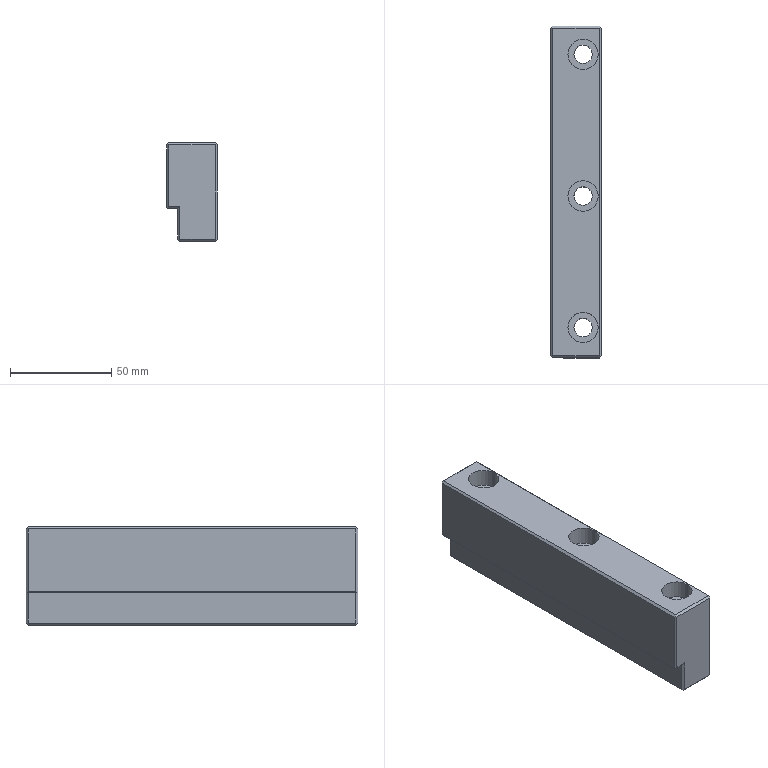Part | Creo | 1 solid | 40 faces | box 25 x 164 x 48.5 mm | volume 171619 mm3 | plane 28 | cylinder 12 | commonest cylinder face diameters 9 x6 15 x6
STEP:
#1=CARTESIAN_POINT('',(99.258,-211.005,-58.5));
#2=VERTEX_POINT('',#1);
#3=CARTESIAN_POINT('',(99.258,-211.005,-12.));
#4=VERTEX_POINT('',#3);
#5=CARTESIAN_POINT('',(99.258,-211.005,-58.5));
#6=DIRECTION('',(0.,0.,1.));
#7=VECTOR('',#6,46.5);
#8=LINE('',#5,#7);
#9=EDGE_CURVE('',#2,#4,#8,.T.);
#10=ORIENTED_EDGE('',*,*,#9,.T.);
#11=CARTESIAN_POINT('',(76.258,-211.005,-12.));
#12=VERTEX_POINT('',#11);
#13=CARTESIAN_POINT('',(99.258,-211.005,-12.));
#14=DIRECTION('',(-1.,0.,0.));
#15=VECTOR('',#14,23.);
#16=LINE('',#13,#15);
#17=EDGE_CURVE('',#4,#12,#16,.T.);
#18=ORIENTED_EDGE('',*,*,#17,.T.);
#19=CARTESIAN_POINT('',(76.258,-211.005,-42.5));
#20=VERTEX_POINT('',#19);
#21=CARTESIAN_POINT('',(76.258,-211.005,-12.));
#22=DIRECTION('',(0.,0.,-1.));
#23=VECTOR('',#22,30.5);
#24=LINE('',#21,#23);
#25=EDGE_CURVE('',#12,#20,#24,.T.);
#26=ORIENTED_EDGE('',*,*,#25,.T.);
#27=CARTESIAN_POINT('',(81.758,-211.005,-42.5));
#28=VERTEX_POINT('',#27);
#29=CARTESIAN_POINT('',(76.258,-211.005,-42.5));
#30=DIRECTION('',(1.,0.,0.));
#31=VECTOR('',#30,5.5);
#32=LINE('',#29,#31);
#33=EDGE_CURVE('',#20,#28,#32,.T.);
#34=ORIENTED_EDGE('',*,*,#33,.T.);
#35=CARTESIAN_POINT('',(81.758,-211.005,-58.5));
#36=VERTEX_POINT('',#35);
#37=CARTESIAN_POINT('',(81.758,-211.005,-42.5));
#38=DIRECTION('',(0.,0.,-1.));
#39=VECTOR('',#38,16.);
#40=LINE('',#37,#39);
#41=EDGE_CURVE('',#28,#36,#40,.T.);
#42=ORIENTED_EDGE('',*,*,#41,.T.);
#43=CARTESIAN_POINT('',(81.758,-211.005,-58.5));
#44=DIRECTION('',(1.,0.,0.));
#45=VECTOR('',#44,17.5);
#46=LINE('',#43,#45);
#47=EDGE_CURVE('',#36,#2,#46,.T.);
#48=ORIENTED_EDGE('',*,*,#47,.T.);
#49=EDGE_LOOP('',(#10,#18,#26,#34,#42,#48));
#50=FACE_OUTER_BOUND('',#49,.F.);
#51=CARTESIAN_POINT('',(-80.242,-211.005,-41.));
#52=DIRECTION('',(0.,1.,0.));
#53=DIRECTION('',(0.,0.,-1.));
#54=AXIS2_PLACEMENT_3D('',#51,#52,#53);
#55=PLANE('',#54);
#56=ADVANCED_FACE('',(#50),#55,.T.);
#57=CARTESIAN_POINT('',(100.258,-212.005,-12.));
#58=VERTEX_POINT('',#57);
#59=CARTESIAN_POINT('',(100.258,-212.005,-58.5));
#60=VERTEX_POINT('',#59);
#61=CARTESIAN_POINT('',(100.258,-212.005,-12.));
#62=DIRECTION('',(0.,0.,-1.));
#63=VECTOR('',#62,46.5);
#64=LINE('',#61,#63);
#65=EDGE_CURVE('',#58,#60,#64,.T.);
#66=ORIENTED_EDGE('',*,*,#65,.F.);
#67=CARTESIAN_POINT('',(99.758,-211.505,-11.5));
#68=VERTEX_POINT('',#67);
#69=CARTESIAN_POINT('',(99.758,-211.505,-11.5));
#70=DIRECTION('',(0.5774,-0.5774,-0.5774));
#71=VECTOR('',#70,0.866);
#72=LINE('',#69,#71);
#73=EDGE_CURVE('',#68,#58,#72,.T.);
#74=ORIENTED_EDGE('',*,*,#73,.F.);
#75=CARTESIAN_POINT('',(99.758,-211.505,-11.5));
#76=DIRECTION('',(-0.5774,0.5774,-0.5774));
#77=VECTOR('',#76,0.866);
#78=LINE('',#75,#77);
#79=EDGE_CURVE('',#68,#4,#78,.T.);
#80=ORIENTED_EDGE('',*,*,#79,.T.);
#81=ORIENTED_EDGE('',*,*,#9,.F.);
#82=CARTESIAN_POINT('',(99.758,-211.505,-59.));
#83=VERTEX_POINT('',#82);
#84=CARTESIAN_POINT('',(99.758,-211.505,-59.));
#85=DIRECTION('',(-0.5774,0.5774,0.5774));
#86=VECTOR('',#85,0.866);
#87=LINE('',#84,#86);
#88=EDGE_CURVE('',#83,#2,#87,.T.);
#89=ORIENTED_EDGE('',*,*,#88,.F.);
#90=CARTESIAN_POINT('',(100.258,-212.005,-58.5));
#91=DIRECTION('',(-0.5774,0.5774,-0.5774));
#92=VECTOR('',#91,0.866);
#93=LINE('',#90,#92);
#94=EDGE_CURVE('',#60,#83,#93,.T.);
#95=ORIENTED_EDGE('',*,*,#94,.F.);
#96=EDGE_LOOP('',(#66,#74,#80,#81,#89,#95));
#97=FACE_OUTER_BOUND('',#96,.F.);
#98=CARTESIAN_POINT('',(99.258,-211.005,-41.));
#99=DIRECTION('',(-0.7071,-0.7071,0.));
#100=DIRECTION('',(0.,0.,-1.));
#101=AXIS2_PLACEMENT_3D('',#98,#99,#100);
#102=PLANE('',#101);
#103=ADVANCED_FACE('',(#97),#102,.F.);
#104=CARTESIAN_POINT('',(100.258,-374.005,-58.5));
#105=VERTEX_POINT('',#104);
#106=CARTESIAN_POINT('',(100.258,-212.005,-58.5));
#107=DIRECTION('',(0.,-1.,0.));
#108=VECTOR('',#107,162.);
#109=LINE('',#106,#108);
#110=EDGE_CURVE('',#60,#105,#109,.T.);
#111=ORIENTED_EDGE('',*,*,#110,.T.);
#112=CARTESIAN_POINT('',(100.258,-374.005,-12.));
#113=VERTEX_POINT('',#112);
#114=CARTESIAN_POINT('',(100.258,-374.005,-12.));
#115=DIRECTION('',(0.,0.,-1.));
#116=VECTOR('',#115,46.5);
#117=LINE('',#114,#116);
#118=EDGE_CURVE('',#113,#105,#117,.T.);
#119=ORIENTED_EDGE('',*,*,#118,.F.);
#120=CARTESIAN_POINT('',(100.258,-212.005,-12.));
#121=DIRECTION('',(0.,-1.,0.));
#122=VECTOR('',#121,162.);
#123=LINE('',#120,#122);
#124=EDGE_CURVE('',#58,#113,#123,.T.);
#125=ORIENTED_EDGE('',*,*,#124,.F.);
#126=ORIENTED_EDGE('',*,*,#65,.T.);
#127=EDGE_LOOP('',(#111,#119,#125,#126));
#128=FACE_OUTER_BOUND('',#127,.F.);
#129=CARTESIAN_POINT('',(100.258,-210.005,-57.));
#130=DIRECTION('',(1.,0.,0.));
#131=DIRECTION('',(0.,0.,-1.));
#132=AXIS2_PLACEMENT_3D('',#129,#130,#131);
#133=PLANE('',#132);
#134=ADVANCED_FACE('',(#128),#133,.T.);
#135=CARTESIAN_POINT('',(99.258,-212.005,-59.5));
#136=VERTEX_POINT('',#135);
#137=CARTESIAN_POINT('',(99.758,-211.505,-59.));
#138=DIRECTION('',(-0.5774,-0.5774,-0.5774));
#139=VECTOR('',#138,0.866);
#140=LINE('',#137,#139);
#141=EDGE_CURVE('',#83,#136,#140,.T.);
#142=ORIENTED_EDGE('',*,*,#141,.T.);
#143=CARTESIAN_POINT('',(99.258,-374.005,-59.5));
#144=VERTEX_POINT('',#143);
#145=CARTESIAN_POINT('',(99.258,-212.005,-59.5));
#146=DIRECTION('',(0.,-1.,0.));
#147=VECTOR('',#146,162.);
#148=LINE('',#145,#147);
#149=EDGE_CURVE('',#136,#144,#148,.T.);
#150=ORIENTED_EDGE('',*,*,#149,.T.);
#151=CARTESIAN_POINT('',(99.758,-374.505,-59.));
#152=VERTEX_POINT('',#151);
#153=CARTESIAN_POINT('',(99.758,-374.505,-59.));
#154=DIRECTION('',(-0.5774,0.5774,-0.5774));
#155=VECTOR('',#154,0.866);
#156=LINE('',#153,#155);
#157=EDGE_CURVE('',#152,#144,#156,.T.);
#158=ORIENTED_EDGE('',*,*,#157,.F.);
#159=CARTESIAN_POINT('',(99.758,-374.505,-59.));
#160=DIRECTION('',(0.5774,0.5774,0.5774));
#161=VECTOR('',#160,0.866);
#162=LINE('',#159,#161);
#163=EDGE_CURVE('',#152,#105,#162,.T.);
#164=ORIENTED_EDGE('',*,*,#163,.T.);
#165=ORIENTED_EDGE('',*,*,#110,.F.);
#166=ORIENTED_EDGE('',*,*,#94,.T.);
#167=EDGE_LOOP('',(#142,#150,#158,#164,#165,#166));
#168=FACE_OUTER_BOUND('',#167,.F.);
#169=CARTESIAN_POINT('',(99.758,-280.005,-59.));
#170=DIRECTION('',(0.7071,0.,-0.7071));
#171=DIRECTION('',(0.7071,0.,0.7071));
#172=AXIS2_PLACEMENT_3D('',#169,#170,#171);
#173=PLANE('',#172);
#174=ADVANCED_FACE('',(#168),#173,.T.);
#175=CARTESIAN_POINT('',(81.758,-212.005,-59.5));
#176=VERTEX_POINT('',#175);
#177=CARTESIAN_POINT('',(99.258,-212.005,-59.5));
#178=DIRECTION('',(-1.,0.,0.));
#179=VECTOR('',#178,17.5);
#180=LINE('',#177,#179);
#181=EDGE_CURVE('',#136,#176,#180,.T.);
#182=ORIENTED_EDGE('',*,*,#181,.F.);
#183=ORIENTED_EDGE('',*,*,#141,.F.);
#184=ORIENTED_EDGE('',*,*,#88,.T.);
#185=ORIENTED_EDGE('',*,*,#47,.F.);
#186=CARTESIAN_POINT('',(81.258,-211.505,-59.));
#187=VERTEX_POINT('',#186);
#188=CARTESIAN_POINT('',(81.258,-211.505,-59.));
#189=DIRECTION('',(0.5774,0.5774,0.5774));
#190=VECTOR('',#189,0.866);
#191=LINE('',#188,#190);
#192=EDGE_CURVE('',#187,#36,#191,.T.);
#193=ORIENTED_EDGE('',*,*,#192,.F.);
#194=CARTESIAN_POINT('',(81.758,-212.005,-59.5));
#195=DIRECTION('',(-0.5774,0.5774,0.5774));
#196=VECTOR('',#195,0.866);
#197=LINE('',#194,#196);
#198=EDGE_CURVE('',#176,#187,#197,.T.);
#199=ORIENTED_EDGE('',*,*,#198,.F.);
#200=EDGE_LOOP('',(#182,#183,#184,#185,#193,#199));
#201=FACE_OUTER_BOUND('',#200,.F.);
#202=CARTESIAN_POINT('',(-80.242,-211.005,-58.5));
#203=DIRECTION('',(0.,-0.7071,0.7071));
#204=DIRECTION('',(-1.,0.,0.));
#205=AXIS2_PLACEMENT_3D('',#202,#203,#204);
#206=PLANE('',#205);
#207=ADVANCED_FACE('',(#201),#206,.F.);
#208=CARTESIAN_POINT('',(81.758,-374.005,-59.5));
#209=VERTEX_POINT('',#208);
#210=CARTESIAN_POINT('',(81.758,-212.005,-59.5));
#211=DIRECTION('',(0.,-1.,0.));
#212=VECTOR('',#211,162.);
#213=LINE('',#210,#212);
#214=EDGE_CURVE('',#176,#209,#213,.T.);
#215=ORIENTED_EDGE('',*,*,#214,.T.);
#216=CARTESIAN_POINT('',(99.258,-374.005,-59.5));
#217=DIRECTION('',(-1.,0.,0.));
#218=VECTOR('',#217,17.5);
#219=LINE('',#216,#218);
#220=EDGE_CURVE('',#144,#209,#219,.T.);
#221=ORIENTED_EDGE('',*,*,#220,.F.);
#222=ORIENTED_EDGE('',*,*,#149,.F.);
#223=ORIENTED_EDGE('',*,*,#181,.T.);
#224=EDGE_LOOP('',(#215,#221,#222,#223));
#225=FACE_OUTER_BOUND('',#224,.F.);
#226=CARTESIAN_POINT('',(86.758,-360.005,-59.5));
#227=VERTEX_POINT('',#226);
#228=CARTESIAN_POINT('',(95.758,-360.005,-59.5));
#229=VERTEX_POINT('',#228);
#230=CARTESIAN_POINT('',(91.258,-360.005,-59.5));
#231=DIRECTION('',(0.,0.,1.));
#232=DIRECTION('',(-1.,0.,0.));
#233=AXIS2_PLACEMENT_3D('',#230,#231,#232);
#234=CIRCLE('',#233,4.5);
#235=EDGE_CURVE('',#227,#229,#234,.T.);
#236=ORIENTED_EDGE('',*,*,#235,.F.);
#237=CARTESIAN_POINT('',(91.258,-360.005,-59.5));
#238=DIRECTION('',(0.,0.,1.));
#239=DIRECTION('',(1.,0.,0.));
#240=AXIS2_PLACEMENT_3D('',#237,#238,#239);
#241=CIRCLE('',#240,4.5);
#242=EDGE_CURVE('',#229,#227,#241,.T.);
#243=ORIENTED_EDGE('',*,*,#242,.F.);
#244=EDGE_LOOP('',(#236,#243));
#245=FACE_BOUND('',#244,.F.);
#246=CARTESIAN_POINT('',(86.758,-225.005,-59.5));
#247=VERTEX_POINT('',#246);
#248=CARTESIAN_POINT('',(95.758,-225.005,-59.5));
#249=VERTEX_POINT('',#248);
#250=CARTESIAN_POINT('',(91.258,-225.005,-59.5));
#251=DIRECTION('',(0.,0.,1.));
#252=DIRECTION('',(-1.,0.,0.));
#253=AXIS2_PLACEMENT_3D('',#250,#251,#252);
#254=CIRCLE('',#253,4.5);
#255=EDGE_CURVE('',#247,#249,#254,.T.);
#256=ORIENTED_EDGE('',*,*,#255,.F.);
#257=CARTESIAN_POINT('',(91.258,-225.005,-59.5));
#258=DIRECTION('',(0.,0.,1.));
#259=DIRECTION('',(1.,0.,0.));
#260=AXIS2_PLACEMENT_3D('',#257,#258,#259);
#261=CIRCLE('',#260,4.5);
#262=EDGE_CURVE('',#249,#247,#261,.T.);
#263=ORIENTED_EDGE('',*,*,#262,.F.);
#264=EDGE_LOOP('',(#256,#263));
#265=FACE_BOUND('',#264,.F.);
#266=CARTESIAN_POINT('',(86.758,-295.005,-59.5));
#267=VERTEX_POINT('',#266);
#268=CARTESIAN_POINT('',(95.758,-295.005,-59.5));
#269=VERTEX_POINT('',#268);
#270=CARTESIAN_POINT('',(91.258,-295.005,-59.5));
#271=DIRECTION('',(0.,0.,1.));
#272=DIRECTION('',(-1.,0.,0.));
#273=AXIS2_PLACEMENT_3D('',#270,#271,#272);
#274=CIRCLE('',#273,4.5);
#275=EDGE_CURVE('',#267,#269,#274,.T.);
#276=ORIENTED_EDGE('',*,*,#275,.F.);
#277=CARTESIAN_POINT('',(91.258,-295.005,-59.5));
#278=DIRECTION('',(0.,0.,1.));
#279=DIRECTION('',(1.,0.,0.));
#280=AXIS2_PLACEMENT_3D('',#277,#278,#279);
#281=CIRCLE('',#280,4.5);
#282=EDGE_CURVE('',#269,#267,#281,.T.);
#283=ORIENTED_EDGE('',*,*,#282,.F.);
#284=EDGE_LOOP('',(#276,#283));
#285=FACE_BOUND('',#284,.F.);
#286=CARTESIAN_POINT('',(80.758,-210.005,-59.5));
#287=DIRECTION('',(0.,0.,-1.));
#288=DIRECTION('',(-1.,0.,0.));
#289=AXIS2_PLACEMENT_3D('',#286,#287,#288);
#290=PLANE('',#289);
#291=ADVANCED_FACE('',(#225,#245,#265,#285),#290,.T.);
#292=CARTESIAN_POINT('',(95.758,-295.005,-20.));
#293=VERTEX_POINT('',#292);
#294=CARTESIAN_POINT('',(86.758,-295.005,-20.));
#295=VERTEX_POINT('',#294);
#296=CARTESIAN_POINT('',(91.258,-295.005,-20.));
#297=DIRECTION('',(0.,0.,-1.));
#298=DIRECTION('',(1.,0.,0.));
#299=AXIS2_PLACEMENT_3D('',#296,#297,#298);
#300=CIRCLE('',#299,4.5);
#301=EDGE_CURVE('',#293,#295,#300,.T.);
#302=ORIENTED_EDGE('',*,*,#301,.T.);
#303=CARTESIAN_POINT('',(86.758,-295.005,-59.5));
#304=DIRECTION('',(0.,0.,1.));
#305=VECTOR('',#304,39.5);
#306=LINE('',#303,#305);
#307=EDGE_CURVE('',#267,#295,#306,.T.);
#308=ORIENTED_EDGE('',*,*,#307,.F.);
#309=ORIENTED_EDGE('',*,*,#275,.T.);
#310=CARTESIAN_POINT('',(95.758,-295.005,-59.5));
#311=DIRECTION('',(0.,0.,1.));
#312=VECTOR('',#311,39.5);
#313=LINE('',#310,#312);
#314=EDGE_CURVE('',#269,#293,#313,.T.);
#315=ORIENTED_EDGE('',*,*,#314,.T.);
#316=EDGE_LOOP('',(#302,#308,#309,#315));
#317=FACE_OUTER_BOUND('',#316,.F.);
#318=CARTESIAN_POINT('',(91.258,-295.005,-10.));
#319=DIRECTION('',(0.,0.,1.));
#320=DIRECTION('',(-1.,0.,0.));
#321=AXIS2_PLACEMENT_3D('',#318,#319,#320);
#322=CYLINDRICAL_SURFACE('',#321,4.5);
#323=ADVANCED_FACE('',(#317),#322,.F.);
#324=CARTESIAN_POINT('',(98.758,-295.005,-20.));
#325=VERTEX_POINT('',#324);
#326=CARTESIAN_POINT('',(83.758,-295.005,-20.));
#327=VERTEX_POINT('',#326);
#328=CARTESIAN_POINT('',(91.258,-295.005,-20.));
#329=DIRECTION('',(0.,0.,1.));
#330=DIRECTION('',(1.,0.,0.));
#331=AXIS2_PLACEMENT_3D('',#328,#329,#330);
#332=CIRCLE('',#331,7.5);
#333=EDGE_CURVE('',#325,#327,#332,.T.);
#334=ORIENTED_EDGE('',*,*,#333,.F.);
#335=CARTESIAN_POINT('',(91.258,-295.005,-20.));
#336=DIRECTION('',(0.,0.,1.));
#337=DIRECTION('',(-1.,0.,0.));
#338=AXIS2_PLACEMENT_3D('',#335,#336,#337);
#339=CIRCLE('',#338,7.5);
#340=EDGE_CURVE('',#327,#325,#339,.T.);
#341=ORIENTED_EDGE('',*,*,#340,.F.);
#342=EDGE_LOOP('',(#334,#341));
#343=FACE_OUTER_BOUND('',#342,.F.);
#344=CARTESIAN_POINT('',(91.258,-295.005,-20.));
#345=DIRECTION('',(0.,0.,-1.));
#346=DIRECTION('',(-1.,0.,0.));
#347=AXIS2_PLACEMENT_3D('',#344,#345,#346);
#348=CIRCLE('',#347,4.5);
#349=EDGE_CURVE('',#295,#293,#348,.T.);
#350=ORIENTED_EDGE('',*,*,#349,.F.);
#351=ORIENTED_EDGE('',*,*,#301,.F.);
#352=EDGE_LOOP('',(#350,#351));
#353=FACE_BOUND('',#352,.F.);
#354=CARTESIAN_POINT('',(91.258,-295.005,-20.));
#355=DIRECTION('',(0.,0.,-1.));
#356=DIRECTION('',(-1.,0.,0.));
#357=AXIS2_PLACEMENT_3D('',#354,#355,#356);
#358=PLANE('',#357);
#359=ADVANCED_FACE('',(#343,#353),#358,.F.);
#360=ORIENTED_EDGE('',*,*,#349,.T.);
#361=ORIENTED_EDGE('',*,*,#314,.F.);
#362=ORIENTED_EDGE('',*,*,#282,.T.);
#363=ORIENTED_EDGE('',*,*,#307,.T.);
#364=EDGE_LOOP('',(#360,#361,#362,#363));
#365=FACE_OUTER_BOUND('',#364,.F.);
#366=CARTESIAN_POINT('',(91.258,-295.005,-10.));
#367=DIRECTION('',(0.,0.,1.));
#368=DIRECTION('',(-1.,0.,0.));
#369=AXIS2_PLACEMENT_3D('',#366,#367,#368);
#370=CYLINDRICAL_SURFACE('',#369,4.5);
#371=ADVANCED_FACE('',(#365),#370,.F.);
#372=ORIENTED_EDGE('',*,*,#333,.T.);
#373=CARTESIAN_POINT('',(83.758,-295.005,-11.));
#374=VERTEX_POINT('',#373);
#375=CARTESIAN_POINT('',(83.758,-295.005,-11.));
#376=DIRECTION('',(0.,0.,-1.));
#377=VECTOR('',#376,9.);
#378=LINE('',#375,#377);
#379=EDGE_CURVE('',#374,#327,#378,.T.);
#380=ORIENTED_EDGE('',*,*,#379,.F.);
#381=CARTESIAN_POINT('',(98.758,-295.005,-11.));
#382=VERTEX_POINT('',#381);
#383=CARTESIAN_POINT('',(91.258,-295.005,-11.));
#384=DIRECTION('',(0.,0.,-1.));
#385=DIRECTION('',(-1.,0.,0.));
#386=AXIS2_PLACEMENT_3D('',#383,#384,#385);
#387=CIRCLE('',#386,7.5);
#388=EDGE_CURVE('',#374,#382,#387,.T.);
#389=ORIENTED_EDGE('',*,*,#388,.T.);
#390=CARTESIAN_POINT('',(98.758,-295.005,-11.));
#391=DIRECTION('',(0.,0.,-1.));
#392=VECTOR('',#391,9.);
#393=LINE('',#390,#392);
#394=EDGE_CURVE('',#382,#325,#393,.T.);
#395=ORIENTED_EDGE('',*,*,#394,.T.);
#396=EDGE_LOOP('',(#372,#380,#389,#395));
#397=FACE_OUTER_BOUND('',#396,.F.);
#398=CARTESIAN_POINT('',(91.258,-295.005,-10.55));
#399=DIRECTION('',(0.,0.,-1.));
#400=DIRECTION('',(-1.,0.,0.));
#401=AXIS2_PLACEMENT_3D('',#398,#399,#400);
#402=CYLINDRICAL_SURFACE('',#401,7.5);
#403=ADVANCED_FACE('',(#397),#402,.F.);
#404=ORIENTED_EDGE('',*,*,#340,.T.);
#405=ORIENTED_EDGE('',*,*,#394,.F.);
#406=CARTESIAN_POINT('',(91.258,-295.005,-11.));
#407=DIRECTION('',(0.,0.,-1.));
#408=DIRECTION('',(1.,0.,0.));
#409=AXIS2_PLACEMENT_3D('',#406,#407,#408);
#410=CIRCLE('',#409,7.5);
#411=EDGE_CURVE('',#382,#374,#410,.T.);
#412=ORIENTED_EDGE('',*,*,#411,.T.);
#413=ORIENTED_EDGE('',*,*,#379,.T.);
#414=EDGE_LOOP('',(#404,#405,#412,#413));
#415=FACE_OUTER_BOUND('',#414,.F.);
#416=CARTESIAN_POINT('',(91.258,-295.005,-10.55));
#417=DIRECTION('',(0.,0.,-1.));
#418=DIRECTION('',(-1.,0.,0.));
#419=AXIS2_PLACEMENT_3D('',#416,#417,#418);
#420=CYLINDRICAL_SURFACE('',#419,7.5);
#421=ADVANCED_FACE('',(#415),#420,.F.);
#422=CARTESIAN_POINT('',(99.258,-212.005,-11.));
#423=VERTEX_POINT('',#422);
#424=CARTESIAN_POINT('',(99.258,-374.005,-11.));
#425=VERTEX_POINT('',#424);
#426=CARTESIAN_POINT('',(99.258,-212.005,-11.));
#427=DIRECTION('',(0.,-1.,0.));
#428=VECTOR('',#427,162.);
#429=LINE('',#426,#428);
#430=EDGE_CURVE('',#423,#425,#429,.T.);
#431=ORIENTED_EDGE('',*,*,#430,.T.);
#432=CARTESIAN_POINT('',(76.258,-374.005,-11.));
#433=VERTEX_POINT('',#432);
#434=CARTESIAN_POINT('',(76.258,-374.005,-11.));
#435=DIRECTION('',(1.,0.,0.));
#436=VECTOR('',#435,23.);
#437=LINE('',#434,#436);
#438=EDGE_CURVE('',#433,#425,#437,.T.);
#439=ORIENTED_EDGE('',*,*,#438,.F.);
#440=CARTESIAN_POINT('',(76.258,-212.005,-11.));
#441=VERTEX_POINT('',#440);
#442=CARTESIAN_POINT('',(76.258,-212.005,-11.));
#443=DIRECTION('',(0.,-1.,0.));
#444=VECTOR('',#443,162.);
#445=LINE('',#442,#444);
#446=EDGE_CURVE('',#441,#433,#445,.T.);
#447=ORIENTED_EDGE('',*,*,#446,.F.);
#448=CARTESIAN_POINT('',(76.258,-212.005,-11.));
#449=DIRECTION('',(1.,0.,0.));
#450=VECTOR('',#449,23.);
#451=LINE('',#448,#450);
#452=EDGE_CURVE('',#441,#423,#451,.T.);
#453=ORIENTED_EDGE('',*,*,#452,.T.);
#454=EDGE_LOOP('',(#431,#439,#447,#453));
#455=FACE_OUTER_BOUND('',#454,.F.);
#456=CARTESIAN_POINT('',(83.758,-360.005,-11.));
#457=VERTEX_POINT('',#456);
#458=CARTESIAN_POINT('',(98.758,-360.005,-11.));
#459=VERTEX_POINT('',#458);
#460=CARTESIAN_POINT('',(91.258,-360.005,-11.));
#461=DIRECTION('',(0.,0.,-1.));
#462=DIRECTION('',(-1.,0.,0.));
#463=AXIS2_PLACEMENT_3D('',#460,#461,#462);
#464=CIRCLE('',#463,7.5);
#465=EDGE_CURVE('',#457,#459,#464,.T.);
#466=ORIENTED_EDGE('',*,*,#465,.F.);
#467=CARTESIAN_POINT('',(91.258,-360.005,-11.));
#468=DIRECTION('',(0.,0.,-1.));
#469=DIRECTION('',(1.,0.,0.));
#470=AXIS2_PLACEMENT_3D('',#467,#468,#469);
#471=CIRCLE('',#470,7.5);
#472=EDGE_CURVE('',#459,#457,#471,.T.);
#473=ORIENTED_EDGE('',*,*,#472,.F.);
#474=EDGE_LOOP('',(#466,#473));
#475=FACE_BOUND('',#474,.F.);
#476=CARTESIAN_POINT('',(83.758,-225.005,-11.));
#477=VERTEX_POINT('',#476);
#478=CARTESIAN_POINT('',(98.758,-225.005,-11.));
#479=VERTEX_POINT('',#478);
#480=CARTESIAN_POINT('',(91.258,-225.005,-11.));
#481=DIRECTION('',(0.,0.,-1.));
#482=DIRECTION('',(-1.,0.,0.));
#483=AXIS2_PLACEMENT_3D('',#480,#481,#482);
#484=CIRCLE('',#483,7.5);
#485=EDGE_CURVE('',#477,#479,#484,.T.);
#486=ORIENTED_EDGE('',*,*,#485,.F.);
#487=CARTESIAN_POINT('',(91.258,-225.005,-11.));
#488=DIRECTION('',(0.,0.,-1.));
#489=DIRECTION('',(1.,0.,0.));
#490=AXIS2_PLACEMENT_3D('',#487,#488,#489);
#491=CIRCLE('',#490,7.5);
#492=EDGE_CURVE('',#479,#477,#491,.T.);
#493=ORIENTED_EDGE('',*,*,#492,.F.);
#494=EDGE_LOOP('',(#486,#493));
#495=FACE_BOUND('',#494,.F.);
#496=ORIENTED_EDGE('',*,*,#388,.F.);
#497=ORIENTED_EDGE('',*,*,#411,.F.);
#498=EDGE_LOOP('',(#496,#497));
#499=FACE_BOUND('',#498,.F.);
#500=CARTESIAN_POINT('',(100.258,-210.005,-11.));
#501=DIRECTION('',(0.,0.,1.));
#502=DIRECTION('',(1.,0.,0.));
#503=AXIS2_PLACEMENT_3D('',#500,#501,#502);
#504=PLANE('',#503);
#505=ADVANCED_FACE('',(#455,#475,#495,#499),#504,.T.);
#506=CARTESIAN_POINT('',(98.758,-360.005,-20.));
#507=VERTEX_POINT('',#506);
#508=CARTESIAN_POINT('',(83.758,-360.005,-20.));
#509=VERTEX_POINT('',#508);
#510=CARTESIAN_POINT('',(91.258,-360.005,-20.));
#511=DIRECTION('',(0.,0.,1.));
#512=DIRECTION('',(1.,0.,0.));
#513=AXIS2_PLACEMENT_3D('',#510,#511,#512);
#514=CIRCLE('',#513,7.5);
#515=EDGE_CURVE('',#507,#509,#514,.T.);
#516=ORIENTED_EDGE('',*,*,#515,.T.);
#517=CARTESIAN_POINT('',(83.758,-360.005,-11.));
#518=DIRECTION('',(0.,0.,-1.));
#519=VECTOR('',#518,9.);
#520=LINE('',#517,#519);
#521=EDGE_CURVE('',#457,#509,#520,.T.);
#522=ORIENTED_EDGE('',*,*,#521,.F.);
#523=ORIENTED_EDGE('',*,*,#465,.T.);
#524=CARTESIAN_POINT('',(98.758,-360.005,-11.));
#525=DIRECTION('',(0.,0.,-1.));
#526=VECTOR('',#525,9.);
#527=LINE('',#524,#526);
#528=EDGE_CURVE('',#459,#507,#527,.T.);
#529=ORIENTED_EDGE('',*,*,#528,.T.);
#530=EDGE_LOOP('',(#516,#522,#523,#529));
#531=FACE_OUTER_BOUND('',#530,.F.);
#532=CARTESIAN_POINT('',(91.258,-360.005,-10.55));
#533=DIRECTION('',(0.,0.,-1.));
#534=DIRECTION('',(-1.,0.,0.));
#535=AXIS2_PLACEMENT_3D('',#532,#533,#534);
#536=CYLINDRICAL_SURFACE('',#535,7.5);
#537=ADVANCED_FACE('',(#531),#536,.F.);
#538=ORIENTED_EDGE('',*,*,#515,.F.);
#539=CARTESIAN_POINT('',(91.258,-360.005,-20.));
#540=DIRECTION('',(0.,0.,1.));
#541=DIRECTION('',(-1.,0.,0.));
#542=AXIS2_PLACEMENT_3D('',#539,#540,#541);
#543=CIRCLE('',#542,7.5);
#544=EDGE_CURVE('',#509,#507,#543,.T.);
#545=ORIENTED_EDGE('',*,*,#544,.F.);
#546=EDGE_LOOP('',(#538,#545));
#547=FACE_OUTER_BOUND('',#546,.F.);
#548=CARTESIAN_POINT('',(86.758,-360.005,-20.));
#549=VERTEX_POINT('',#548);
#550=CARTESIAN_POINT('',(95.758,-360.005,-20.));
#551=VERTEX_POINT('',#550);
#552=CARTESIAN_POINT('',(91.258,-360.005,-20.));
#553=DIRECTION('',(0.,0.,-1.));
#554=DIRECTION('',(-1.,0.,0.));
#555=AXIS2_PLACEMENT_3D('',#552,#553,#554);
#556=CIRCLE('',#555,4.5);
#557=EDGE_CURVE('',#549,#551,#556,.T.);
#558=ORIENTED_EDGE('',*,*,#557,.F.);
#559=CARTESIAN_POINT('',(91.258,-360.005,-20.));
#560=DIRECTION('',(0.,0.,-1.));
#561=DIRECTION('',(1.,0.,0.));
#562=AXIS2_PLACEMENT_3D('',#559,#560,#561);
#563=CIRCLE('',#562,4.5);
#564=EDGE_CURVE('',#551,#549,#563,.T.);
#565=ORIENTED_EDGE('',*,*,#564,.F.);
#566=EDGE_LOOP('',(#558,#565));
#567=FACE_BOUND('',#566,.F.);
#568=CARTESIAN_POINT('',(91.258,-360.005,-20.));
#569=DIRECTION('',(0.,0.,-1.));
#570=DIRECTION('',(-1.,0.,0.));
#571=AXIS2_PLACEMENT_3D('',#568,#569,#570);
#572=PLANE('',#571);
#573=ADVANCED_FACE('',(#547,#567),#572,.F.);
#574=ORIENTED_EDGE('',*,*,#557,.T.);
#575=CARTESIAN_POINT('',(95.758,-360.005,-59.5));
#576=DIRECTION('',(0.,0.,1.));
#577=VECTOR('',#576,39.5);
#578=LINE('',#575,#577);
#579=EDGE_CURVE('',#229,#551,#578,.T.);
#580=ORIENTED_EDGE('',*,*,#579,.F.);
#581=ORIENTED_EDGE('',*,*,#242,.T.);
#582=CARTESIAN_POINT('',(86.758,-360.005,-59.5));
#583=DIRECTION('',(0.,0.,1.));
#584=VECTOR('',#583,39.5);
#585=LINE('',#582,#584);
#586=EDGE_CURVE('',#227,#549,#585,.T.);
#587=ORIENTED_EDGE('',*,*,#586,.T.);
#588=EDGE_LOOP('',(#574,#580,#581,#587));
#589=FACE_OUTER_BOUND('',#588,.F.);
#590=CARTESIAN_POINT('',(91.258,-360.005,-10.));
#591=DIRECTION('',(0.,0.,1.));
#592=DIRECTION('',(-1.,0.,0.));
#593=AXIS2_PLACEMENT_3D('',#590,#591,#592);
#594=CYLINDRICAL_SURFACE('',#593,4.5);
#595=ADVANCED_FACE('',(#589),#594,.F.);
#596=ORIENTED_EDGE('',*,*,#564,.T.);
#597=ORIENTED_EDGE('',*,*,#586,.F.);
#598=ORIENTED_EDGE('',*,*,#235,.T.);
#599=ORIENTED_EDGE('',*,*,#579,.T.);
#600=EDGE_LOOP('',(#596,#597,#598,#599));
#601=FACE_OUTER_BOUND('',#600,.F.);
#602=CARTESIAN_POINT('',(91.258,-360.005,-10.));
#603=DIRECTION('',(0.,0.,1.));
#604=DIRECTION('',(-1.,0.,0.));
#605=AXIS2_PLACEMENT_3D('',#602,#603,#604);
#606=CYLINDRICAL_SURFACE('',#605,4.5);
#607=ADVANCED_FACE('',(#601),#606,.F.);
#608=ORIENTED_EDGE('',*,*,#544,.T.);
#609=ORIENTED_EDGE('',*,*,#528,.F.);
#610=ORIENTED_EDGE('',*,*,#472,.T.);
#611=ORIENTED_EDGE('',*,*,#521,.T.);
#612=EDGE_LOOP('',(#608,#609,#610,#611));
#613=FACE_OUTER_BOUND('',#612,.F.);
#614=CARTESIAN_POINT('',(91.258,-360.005,-10.55));
#615=DIRECTION('',(0.,0.,-1.));
#616=DIRECTION('',(-1.,0.,0.));
#617=AXIS2_PLACEMENT_3D('',#614,#615,#616);
#618=CYLINDRICAL_SURFACE('',#617,7.5);
#619=ADVANCED_FACE('',(#613),#618,.F.);
#620=CARTESIAN_POINT('',(98.758,-225.005,-20.));
#621=VERTEX_POINT('',#620);
#622=CARTESIAN_POINT('',(83.758,-225.005,-20.));
#623=VERTEX_POINT('',#622);
#624=CARTESIAN_POINT('',(91.258,-225.005,-20.));
#625=DIRECTION('',(0.,0.,1.));
#626=DIRECTION('',(1.,0.,0.));
#627=AXIS2_PLACEMENT_3D('',#624,#625,#626);
#628=CIRCLE('',#627,7.5);
#629=EDGE_CURVE('',#621,#623,#628,.T.);
#630=ORIENTED_EDGE('',*,*,#629,.T.);
#631=CARTESIAN_POINT('',(83.758,-225.005,-11.));
#632=DIRECTION('',(0.,0.,-1.));
#633=VECTOR('',#632,9.);
#634=LINE('',#631,#633);
#635=EDGE_CURVE('',#477,#623,#634,.T.);
#636=ORIENTED_EDGE('',*,*,#635,.F.);
#637=ORIENTED_EDGE('',*,*,#485,.T.);
#638=CARTESIAN_POINT('',(98.758,-225.005,-11.));
#639=DIRECTION('',(0.,0.,-1.));
#640=VECTOR('',#639,9.);
#641=LINE('',#638,#640);
#642=EDGE_CURVE('',#479,#621,#641,.T.);
#643=ORIENTED_EDGE('',*,*,#642,.T.);
#644=EDGE_LOOP('',(#630,#636,#637,#643));
#645=FACE_OUTER_BOUND('',#644,.F.);
#646=CARTESIAN_POINT('',(91.258,-225.005,-10.55));
#647=DIRECTION('',(0.,0.,-1.));
#648=DIRECTION('',(-1.,0.,0.));
#649=AXIS2_PLACEMENT_3D('',#646,#647,#648);
#650=CYLINDRICAL_SURFACE('',#649,7.5);
#651=ADVANCED_FACE('',(#645),#650,.F.);
#652=ORIENTED_EDGE('',*,*,#629,.F.);
#653=CARTESIAN_POINT('',(91.258,-225.005,-20.));
#654=DIRECTION('',(0.,0.,1.));
#655=DIRECTION('',(-1.,0.,0.));
#656=AXIS2_PLACEMENT_3D('',#653,#654,#655);
#657=CIRCLE('',#656,7.5);
#658=EDGE_CURVE('',#623,#621,#657,.T.);
#659=ORIENTED_EDGE('',*,*,#658,.F.);
#660=EDGE_LOOP('',(#652,#659));
#661=FACE_OUTER_BOUND('',#660,.F.);
#662=CARTESIAN_POINT('',(86.758,-225.005,-20.));
#663=VERTEX_POINT('',#662);
#664=CARTESIAN_POINT('',(95.758,-225.005,-20.));
#665=VERTEX_POINT('',#664);
#666=CARTESIAN_POINT('',(91.258,-225.005,-20.));
#667=DIRECTION('',(0.,0.,-1.));
#668=DIRECTION('',(-1.,0.,0.));
#669=AXIS2_PLACEMENT_3D('',#666,#667,#668);
#670=CIRCLE('',#669,4.5);
#671=EDGE_CURVE('',#663,#665,#670,.T.);
#672=ORIENTED_EDGE('',*,*,#671,.F.);
#673=CARTESIAN_POINT('',(91.258,-225.005,-20.));
#674=DIRECTION('',(0.,0.,-1.));
#675=DIRECTION('',(1.,0.,0.));
#676=AXIS2_PLACEMENT_3D('',#673,#674,#675);
#677=CIRCLE('',#676,4.5);
#678=EDGE_CURVE('',#665,#663,#677,.T.);
#679=ORIENTED_EDGE('',*,*,#678,.F.);
#680=EDGE_LOOP('',(#672,#679));
#681=FACE_BOUND('',#680,.F.);
#682=CARTESIAN_POINT('',(91.258,-225.005,-20.));
#683=DIRECTION('',(0.,0.,-1.));
#684=DIRECTION('',(-1.,0.,0.));
#685=AXIS2_PLACEMENT_3D('',#682,#683,#684);
#686=PLANE('',#685);
#687=ADVANCED_FACE('',(#661,#681),#686,.F.);
#688=ORIENTED_EDGE('',*,*,#671,.T.);
#689=CARTESIAN_POINT('',(95.758,-225.005,-59.5));
#690=DIRECTION('',(0.,0.,1.));
#691=VECTOR('',#690,39.5);
#692=LINE('',#689,#691);
#693=EDGE_CURVE('',#249,#665,#692,.T.);
#694=ORIENTED_EDGE('',*,*,#693,.F.);
#695=ORIENTED_EDGE('',*,*,#262,.T.);
#696=CARTESIAN_POINT('',(86.758,-225.005,-59.5));
#697=DIRECTION('',(0.,0.,1.));
#698=VECTOR('',#697,39.5);
#699=LINE('',#696,#698);
#700=EDGE_CURVE('',#247,#663,#699,.T.);
#701=ORIENTED_EDGE('',*,*,#700,.T.);
#702=EDGE_LOOP('',(#688,#694,#695,#701));
#703=FACE_OUTER_BOUND('',#702,.F.);
#704=CARTESIAN_POINT('',(91.258,-225.005,-10.));
#705=DIRECTION('',(0.,0.,1.));
#706=DIRECTION('',(-1.,0.,0.));
#707=AXIS2_PLACEMENT_3D('',#704,#705,#706);
#708=CYLINDRICAL_SURFACE('',#707,4.5);
#709=ADVANCED_FACE('',(#703),#708,.F.);
#710=ORIENTED_EDGE('',*,*,#678,.T.);
#711=ORIENTED_EDGE('',*,*,#700,.F.);
#712=ORIENTED_EDGE('',*,*,#255,.T.);
#713=ORIENTED_EDGE('',*,*,#693,.T.);
#714=EDGE_LOOP('',(#710,#711,#712,#713));
#715=FACE_OUTER_BOUND('',#714,.F.);
#716=CARTESIAN_POINT('',(91.258,-225.005,-10.));
#717=DIRECTION('',(0.,0.,1.));
#718=DIRECTION('',(-1.,0.,0.));
#719=AXIS2_PLACEMENT_3D('',#716,#717,#718);
#720=CYLINDRICAL_SURFACE('',#719,4.5);
#721=ADVANCED_FACE('',(#715),#720,.F.);
#722=ORIENTED_EDGE('',*,*,#658,.T.);
#723=ORIENTED_EDGE('',*,*,#642,.F.);
#724=ORIENTED_EDGE('',*,*,#492,.T.);
#725=ORIENTED_EDGE('',*,*,#635,.T.);
#726=EDGE_LOOP('',(#722,#723,#724,#725));
#727=FACE_OUTER_BOUND('',#726,.F.);
#728=CARTESIAN_POINT('',(91.258,-225.005,-10.55));
#729=DIRECTION('',(0.,0.,-1.));
#730=DIRECTION('',(-1.,0.,0.));
#731=AXIS2_PLACEMENT_3D('',#728,#729,#730);
#732=CYLINDRICAL_SURFACE('',#731,7.5);
#733=ADVANCED_FACE('',(#727),#732,.F.);
#734=ORIENTED_EDGE('',*,*,#124,.T.);
#735=CARTESIAN_POINT('',(99.758,-374.505,-11.5));
#736=VERTEX_POINT('',#735);
#737=CARTESIAN_POINT('',(100.258,-374.005,-12.));
#738=DIRECTION('',(-0.5774,-0.5774,0.5774));
#739=VECTOR('',#738,0.866);
#740=LINE('',#737,#739);
#741=EDGE_CURVE('',#113,#736,#740,.T.);
#742=ORIENTED_EDGE('',*,*,#741,.T.);
#743=CARTESIAN_POINT('',(99.758,-374.505,-11.5));
#744=DIRECTION('',(-0.5774,0.5774,0.5774));
#745=VECTOR('',#744,0.866);
#746=LINE('',#743,#745);
#747=EDGE_CURVE('',#736,#425,#746,.T.);
#748=ORIENTED_EDGE('',*,*,#747,.T.);
#749=ORIENTED_EDGE('',*,*,#430,.F.);
#750=CARTESIAN_POINT('',(99.258,-212.005,-11.));
#751=DIRECTION('',(0.5774,0.5774,-0.5774));
#752=VECTOR('',#751,0.866);
#753=LINE('',#750,#752);
#754=EDGE_CURVE('',#423,#68,#753,.T.);
#755=ORIENTED_EDGE('',*,*,#754,.T.);
#756=ORIENTED_EDGE('',*,*,#73,.T.);
#757=EDGE_LOOP('',(#734,#742,#748,#749,#755,#756));
#758=FACE_OUTER_BOUND('',#757,.F.);
#759=CARTESIAN_POINT('',(99.758,-280.005,-11.5));
#760=DIRECTION('',(0.7071,0.,0.7071));
#761=DIRECTION('',(-0.7071,0.,0.7071));
#762=AXIS2_PLACEMENT_3D('',#759,#760,#761);
#763=PLANE('',#762);
#764=ADVANCED_FACE('',(#758),#763,.T.);
#765=ORIENTED_EDGE('',*,*,#741,.F.);
#766=ORIENTED_EDGE('',*,*,#118,.T.);
#767=ORIENTED_EDGE('',*,*,#163,.F.);
#768=CARTESIAN_POINT('',(99.258,-375.005,-58.5));
#769=VERTEX_POINT('',#768);
#770=CARTESIAN_POINT('',(99.258,-375.005,-58.5));
#771=DIRECTION('',(0.5774,0.5774,-0.5774));
#772=VECTOR('',#771,0.866);
#773=LINE('',#770,#772);
#774=EDGE_CURVE('',#769,#152,#773,.T.);
#775=ORIENTED_EDGE('',*,*,#774,.F.);
#776=CARTESIAN_POINT('',(99.258,-375.005,-12.));
#777=VERTEX_POINT('',#776);
#778=CARTESIAN_POINT('',(99.258,-375.005,-12.));
#779=DIRECTION('',(0.,0.,-1.));
#780=VECTOR('',#779,46.5);
#781=LINE('',#778,#780);
#782=EDGE_CURVE('',#777,#769,#781,.T.);
#783=ORIENTED_EDGE('',*,*,#782,.F.);
#784=CARTESIAN_POINT('',(99.758,-374.505,-11.5));
#785=DIRECTION('',(-0.5774,-0.5774,-0.5774));
#786=VECTOR('',#785,0.866);
#787=LINE('',#784,#786);
#788=EDGE_CURVE('',#736,#777,#787,.T.);
#789=ORIENTED_EDGE('',*,*,#788,.F.);
#790=EDGE_LOOP('',(#765,#766,#767,#775,#783,#789));
#791=FACE_OUTER_BOUND('',#790,.F.);
#792=CARTESIAN_POINT('',(99.758,-374.505,-29.));
#793=DIRECTION('',(0.7071,-0.7071,0.));
#794=DIRECTION('',(-0.7071,-0.7071,0.));
#795=AXIS2_PLACEMENT_3D('',#792,#793,#794);
#796=PLANE('',#795);
#797=ADVANCED_FACE('',(#791),#796,.T.);
#798=CARTESIAN_POINT('',(81.258,-374.505,-59.));
#799=VERTEX_POINT('',#798);
#800=CARTESIAN_POINT('',(81.758,-375.005,-58.5));
#801=VERTEX_POINT('',#800);
#802=CARTESIAN_POINT('',(81.258,-374.505,-59.));
#803=DIRECTION('',(0.5774,-0.5774,0.5774));
#804=VECTOR('',#803,0.866);
#805=LINE('',#802,#804);
#806=EDGE_CURVE('',#799,#801,#805,.T.);
#807=ORIENTED_EDGE('',*,*,#806,.T.);
#808=CARTESIAN_POINT('',(99.258,-375.005,-58.5));
#809=DIRECTION('',(-1.,0.,0.));
#810=VECTOR('',#809,17.5);
#811=LINE('',#808,#810);
#812=EDGE_CURVE('',#769,#801,#811,.T.);
#813=ORIENTED_EDGE('',*,*,#812,.F.);
#814=ORIENTED_EDGE('',*,*,#774,.T.);
#815=ORIENTED_EDGE('',*,*,#157,.T.);
#816=ORIENTED_EDGE('',*,*,#220,.T.);
#817=CARTESIAN_POINT('',(81.258,-374.505,-59.));
#818=DIRECTION('',(0.5774,0.5774,-0.5774));
#819=VECTOR('',#818,0.866);
#820=LINE('',#817,#819);
#821=EDGE_CURVE('',#799,#209,#820,.T.);
#822=ORIENTED_EDGE('',*,*,#821,.F.);
#823=EDGE_LOOP('',(#807,#813,#814,#815,#816,#822));
#824=FACE_OUTER_BOUND('',#823,.F.);
#825=CARTESIAN_POINT('',(90.508,-374.505,-59.));
#826=DIRECTION('',(0.,-0.7071,-0.7071));
#827=DIRECTION('',(0.,-0.7071,0.7071));
#828=AXIS2_PLACEMENT_3D('',#825,#826,#827);
#829=PLANE('',#828);
#830=ADVANCED_FACE('',(#824),#829,.T.);
#831=CARTESIAN_POINT('',(80.758,-374.005,-58.5));
#832=VERTEX_POINT('',#831);
#833=CARTESIAN_POINT('',(80.758,-374.005,-58.5));
#834=DIRECTION('',(0.5774,-0.5774,-0.5774));
#835=VECTOR('',#834,0.866);
#836=LINE('',#833,#835);
#837=EDGE_CURVE('',#832,#799,#836,.T.);
#838=ORIENTED_EDGE('',*,*,#837,.F.);
#839=CARTESIAN_POINT('',(80.758,-374.005,-43.5));
#840=VERTEX_POINT('',#839);
#841=CARTESIAN_POINT('',(80.758,-374.005,-58.5));
#842=DIRECTION('',(0.,0.,1.));
#843=VECTOR('',#842,15.);
#844=LINE('',#841,#843);
#845=EDGE_CURVE('',#832,#840,#844,.T.);
#846=ORIENTED_EDGE('',*,*,#845,.T.);
#847=CARTESIAN_POINT('',(81.758,-375.005,-42.5));
#848=VERTEX_POINT('',#847);
#849=CARTESIAN_POINT('',(81.758,-375.005,-42.5));
#850=DIRECTION('',(-0.5774,0.5774,-0.5774));
#851=VECTOR('',#850,1.732);
#852=LINE('',#849,#851);
#853=EDGE_CURVE('',#848,#840,#852,.T.);
#854=ORIENTED_EDGE('',*,*,#853,.F.);
#855=CARTESIAN_POINT('',(81.758,-375.005,-58.5));
#856=DIRECTION('',(0.,0.,1.));
#857=VECTOR('',#856,16.);
#858=LINE('',#855,#857);
#859=EDGE_CURVE('',#801,#848,#858,.T.);
#860=ORIENTED_EDGE('',*,*,#859,.F.);
#861=ORIENTED_EDGE('',*,*,#806,.F.);
#862=EDGE_LOOP('',(#838,#846,#854,#860,#861));
#863=FACE_OUTER_BOUND('',#862,.F.);
#864=CARTESIAN_POINT('',(81.258,-374.505,-51.5));
#865=DIRECTION('',(-0.7071,-0.7071,0.));
#866=DIRECTION('',(0.7071,-0.7071,0.));
#867=AXIS2_PLACEMENT_3D('',#864,#865,#866);
#868=PLANE('',#867);
#869=ADVANCED_FACE('',(#863),#868,.T.);
#870=CARTESIAN_POINT('',(80.758,-212.005,-58.5));
#871=VERTEX_POINT('',#870);
#872=CARTESIAN_POINT('',(80.758,-212.005,-58.5));
#873=DIRECTION('',(0.,-1.,0.));
#874=VECTOR('',#873,162.);
#875=LINE('',#872,#874);
#876=EDGE_CURVE('',#871,#832,#875,.T.);
#877=ORIENTED_EDGE('',*,*,#876,.T.);
#878=ORIENTED_EDGE('',*,*,#837,.T.);
#879=ORIENTED_EDGE('',*,*,#821,.T.);
#880=ORIENTED_EDGE('',*,*,#214,.F.);
#881=ORIENTED_EDGE('',*,*,#198,.T.);
#882=CARTESIAN_POINT('',(81.258,-211.505,-59.));
#883=DIRECTION('',(-0.5774,-0.5774,0.5774));
#884=VECTOR('',#883,0.866);
#885=LINE('',#882,#884);
#886=EDGE_CURVE('',#187,#871,#885,.T.);
#887=ORIENTED_EDGE('',*,*,#886,.T.);
#888=EDGE_LOOP('',(#877,#878,#879,#880,#881,#887));
#889=FACE_OUTER_BOUND('',#888,.F.);
#890=CARTESIAN_POINT('',(81.258,-280.005,-59.));
#891=DIRECTION('',(-0.7071,0.,-0.7071));
#892=DIRECTION('',(0.7071,0.,-0.7071));
#893=AXIS2_PLACEMENT_3D('',#890,#891,#892);
#894=PLANE('',#893);
#895=ADVANCED_FACE('',(#889),#894,.T.);
#896=CARTESIAN_POINT('',(80.758,-212.005,-43.5));
#897=VERTEX_POINT('',#896);
#898=CARTESIAN_POINT('',(80.758,-374.005,-43.5));
#899=DIRECTION('',(0.,1.,0.));
#900=VECTOR('',#899,162.);
#901=LINE('',#898,#900);
#902=EDGE_CURVE('',#840,#897,#901,.T.);
#903=ORIENTED_EDGE('',*,*,#902,.F.);
#904=ORIENTED_EDGE('',*,*,#845,.F.);
#905=ORIENTED_EDGE('',*,*,#876,.F.);
#906=CARTESIAN_POINT('',(80.758,-212.005,-58.5));
#907=DIRECTION('',(0.,0.,1.));
#908=VECTOR('',#907,15.);
#909=LINE('',#906,#908);
#910=EDGE_CURVE('',#871,#897,#909,.T.);
#911=ORIENTED_EDGE('',*,*,#910,.T.);
#912=EDGE_LOOP('',(#903,#904,#905,#911));
#913=FACE_OUTER_BOUND('',#912,.F.);
#914=CARTESIAN_POINT('',(80.758,-210.005,-43.5));
#915=DIRECTION('',(-1.,0.,0.));
#916=DIRECTION('',(0.,0.,1.));
#917=AXIS2_PLACEMENT_3D('',#914,#915,#916);
#918=PLANE('',#917);
#919=ADVANCED_FACE('',(#913),#918,.T.);
#920=CARTESIAN_POINT('',(75.758,-212.005,-43.5));
#921=VERTEX_POINT('',#920);
#922=CARTESIAN_POINT('',(75.758,-374.005,-43.5));
#923=VERTEX_POINT('',#922);
#924=CARTESIAN_POINT('',(75.758,-212.005,-43.5));
#925=DIRECTION('',(0.,-1.,0.));
#926=VECTOR('',#925,162.);
#927=LINE('',#924,#926);
#928=EDGE_CURVE('',#921,#923,#927,.T.);
#929=ORIENTED_EDGE('',*,*,#928,.T.);
#930=CARTESIAN_POINT('',(80.758,-374.005,-43.5));
#931=DIRECTION('',(-1.,0.,0.));
#932=VECTOR('',#931,5.);
#933=LINE('',#930,#932);
#934=EDGE_CURVE('',#840,#923,#933,.T.);
#935=ORIENTED_EDGE('',*,*,#934,.F.);
#936=ORIENTED_EDGE('',*,*,#902,.T.);
#937=CARTESIAN_POINT('',(80.758,-212.005,-43.5));
#938=DIRECTION('',(-1.,0.,0.));
#939=VECTOR('',#938,5.);
#940=LINE('',#937,#939);
#941=EDGE_CURVE('',#897,#921,#940,.T.);
#942=ORIENTED_EDGE('',*,*,#941,.T.);
#943=EDGE_LOOP('',(#929,#935,#936,#942));
#944=FACE_OUTER_BOUND('',#943,.F.);
#945=CARTESIAN_POINT('',(75.258,-210.005,-43.5));
#946=DIRECTION('',(0.,0.,-1.));
#947=DIRECTION('',(-1.,0.,0.));
#948=AXIS2_PLACEMENT_3D('',#945,#946,#947);
#949=PLANE('',#948);
#950=ADVANCED_FACE('',(#944),#949,.T.);
#951=CARTESIAN_POINT('',(75.508,-211.755,-43.25));
#952=VERTEX_POINT('',#951);
#953=CARTESIAN_POINT('',(75.258,-212.005,-43.));
#954=VERTEX_POINT('',#953);
#955=CARTESIAN_POINT('',(75.508,-211.755,-43.25));
#956=DIRECTION('',(-0.5774,-0.5774,0.5774));
#957=VECTOR('',#956,0.433);
#958=LINE('',#955,#957);
#959=EDGE_CURVE('',#952,#954,#958,.T.);
#960=ORIENTED_EDGE('',*,*,#959,.T.);
#961=CARTESIAN_POINT('',(75.258,-374.005,-43.));
#962=VERTEX_POINT('',#961);
#963=CARTESIAN_POINT('',(75.258,-212.005,-43.));
#964=DIRECTION('',(0.,-1.,0.));
#965=VECTOR('',#964,162.);
#966=LINE('',#963,#965);
#967=EDGE_CURVE('',#954,#962,#966,.T.);
#968=ORIENTED_EDGE('',*,*,#967,.T.);
#969=CARTESIAN_POINT('',(75.508,-374.255,-43.25));
#970=VERTEX_POINT('',#969);
#971=CARTESIAN_POINT('',(75.508,-374.255,-43.25));
#972=DIRECTION('',(-0.5774,0.5774,0.5774));
#973=VECTOR('',#972,0.433);
#974=LINE('',#971,#973);
#975=EDGE_CURVE('',#970,#962,#974,.T.);
#976=ORIENTED_EDGE('',*,*,#975,.F.);
#977=CARTESIAN_POINT('',(75.758,-374.005,-43.5));
#978=DIRECTION('',(-0.5774,-0.5774,0.5774));
#979=VECTOR('',#978,0.433);
#980=LINE('',#977,#979);
#981=EDGE_CURVE('',#923,#970,#980,.T.);
#982=ORIENTED_EDGE('',*,*,#981,.F.);
#983=ORIENTED_EDGE('',*,*,#928,.F.);
#984=CARTESIAN_POINT('',(75.758,-212.005,-43.5));
#985=DIRECTION('',(-0.5774,0.5774,0.5774));
#986=VECTOR('',#985,0.433);
#987=LINE('',#984,#986);
#988=EDGE_CURVE('',#921,#952,#987,.T.);
#989=ORIENTED_EDGE('',*,*,#988,.T.);
#990=EDGE_LOOP('',(#960,#968,#976,#982,#983,#989));
#991=FACE_OUTER_BOUND('',#990,.F.);
#992=CARTESIAN_POINT('',(75.508,-280.005,-43.25));
#993=DIRECTION('',(-0.7071,0.,-0.7071));
#994=DIRECTION('',(0.7071,0.,-0.7071));
#995=AXIS2_PLACEMENT_3D('',#992,#993,#994);
#996=PLANE('',#995);
#997=ADVANCED_FACE('',(#991),#996,.T.);
#998=CARTESIAN_POINT('',(75.758,-211.505,-11.5));
#999=VERTEX_POINT('',#998);
#1000=CARTESIAN_POINT('',(76.258,-211.005,-12.));
#1001=DIRECTION('',(-0.5774,-0.5774,0.5774));
#1002=VECTOR('',#1001,0.866);
#1003=LINE('',#1000,#1002);
#1004=EDGE_CURVE('',#12,#999,#1003,.T.);
#1005=ORIENTED_EDGE('',*,*,#1004,.T.);
#1006=CARTESIAN_POINT('',(75.258,-212.005,-12.));
#1007=VERTEX_POINT('',#1006);
#1008=CARTESIAN_POINT('',(75.258,-212.005,-12.));
#1009=DIRECTION('',(0.5774,0.5774,0.5774));
#1010=VECTOR('',#1009,0.866);
#1011=LINE('',#1008,#1010);
#1012=EDGE_CURVE('',#1007,#999,#1011,.T.);
#1013=ORIENTED_EDGE('',*,*,#1012,.F.);
#1014=CARTESIAN_POINT('',(75.258,-212.005,-43.));
#1015=DIRECTION('',(0.,0.,1.));
#1016=VECTOR('',#1015,31.);
#1017=LINE('',#1014,#1016);
#1018=EDGE_CURVE('',#954,#1007,#1017,.T.);
#1019=ORIENTED_EDGE('',*,*,#1018,.F.);
#1020=ORIENTED_EDGE('',*,*,#959,.F.);
#1021=CARTESIAN_POINT('',(76.258,-211.005,-42.5));
#1022=DIRECTION('',(-0.5774,-0.5774,-0.5774));
#1023=VECTOR('',#1022,1.299);
#1024=LINE('',#1021,#1023);
#1025=EDGE_CURVE('',#20,#952,#1024,.T.);
#1026=ORIENTED_EDGE('',*,*,#1025,.F.);
#1027=ORIENTED_EDGE('',*,*,#25,.F.);
#1028=EDGE_LOOP('',(#1005,#1013,#1019,#1020,#1026,#1027));
#1029=FACE_OUTER_BOUND('',#1028,.F.);
#1030=CARTESIAN_POINT('',(76.258,-211.005,-41.));
#1031=DIRECTION('',(0.7071,-0.7071,0.));
#1032=DIRECTION('',(0.,0.,1.));
#1033=AXIS2_PLACEMENT_3D('',#1030,#1031,#1032);
#1034=PLANE('',#1033);
#1035=ADVANCED_FACE('',(#1029),#1034,.F.);
#1036=ORIENTED_EDGE('',*,*,#452,.F.);
#1037=CARTESIAN_POINT('',(75.758,-211.505,-11.5));
#1038=DIRECTION('',(0.5774,-0.5774,0.5774));
#1039=VECTOR('',#1038,0.866);
#1040=LINE('',#1037,#1039);
#1041=EDGE_CURVE('',#999,#441,#1040,.T.);
#1042=ORIENTED_EDGE('',*,*,#1041,.F.);
#1043=ORIENTED_EDGE('',*,*,#1004,.F.);
#1044=ORIENTED_EDGE('',*,*,#17,.F.);
#1045=ORIENTED_EDGE('',*,*,#79,.F.);
#1046=ORIENTED_EDGE('',*,*,#754,.F.);
#1047=EDGE_LOOP('',(#1036,#1042,#1043,#1044,#1045,#1046));
#1048=FACE_OUTER_BOUND('',#1047,.F.);
#1049=CARTESIAN_POINT('',(-80.242,-211.005,-12.));
#1050=DIRECTION('',(0.,-0.7071,-0.7071));
#1051=DIRECTION('',(1.,0.,0.));
#1052=AXIS2_PLACEMENT_3D('',#1049,#1050,#1051);
#1053=PLANE('',#1052);
#1054=ADVANCED_FACE('',(#1048),#1053,.F.);
#1055=ORIENTED_EDGE('',*,*,#1041,.T.);
#1056=ORIENTED_EDGE('',*,*,#446,.T.);
#1057=CARTESIAN_POINT('',(75.758,-374.505,-11.5));
#1058=VERTEX_POINT('',#1057);
#1059=CARTESIAN_POINT('',(75.758,-374.505,-11.5));
#1060=DIRECTION('',(0.5774,0.5774,0.5774));
#1061=VECTOR('',#1060,0.866);
#1062=LINE('',#1059,#1061);
#1063=EDGE_CURVE('',#1058,#433,#1062,.T.);
#1064=ORIENTED_EDGE('',*,*,#1063,.F.);
#1065=CARTESIAN_POINT('',(75.258,-374.005,-12.));
#1066=VERTEX_POINT('',#1065);
#1067=CARTESIAN_POINT('',(75.758,-374.505,-11.5));
#1068=DIRECTION('',(-0.5774,0.5774,-0.5774));
#1069=VECTOR('',#1068,0.866);
#1070=LINE('',#1067,#1069);
#1071=EDGE_CURVE('',#1058,#1066,#1070,.T.);
#1072=ORIENTED_EDGE('',*,*,#1071,.T.);
#1073=CARTESIAN_POINT('',(75.258,-212.005,-12.));
#1074=DIRECTION('',(0.,-1.,0.));
#1075=VECTOR('',#1074,162.);
#1076=LINE('',#1073,#1075);
#1077=EDGE_CURVE('',#1007,#1066,#1076,.T.);
#1078=ORIENTED_EDGE('',*,*,#1077,.F.);
#1079=ORIENTED_EDGE('',*,*,#1012,.T.);
#1080=EDGE_LOOP('',(#1055,#1056,#1064,#1072,#1078,#1079));
#1081=FACE_OUTER_BOUND('',#1080,.F.);
#1082=CARTESIAN_POINT('',(75.758,-280.005,-11.5));
#1083=DIRECTION('',(-0.7071,0.,0.7071));
#1084=DIRECTION('',(-0.7071,0.,-0.7071));
#1085=AXIS2_PLACEMENT_3D('',#1082,#1083,#1084);
#1086=PLANE('',#1085);
#1087=ADVANCED_FACE('',(#1081),#1086,.T.);
#1088=ORIENTED_EDGE('',*,*,#788,.T.);
#1089=CARTESIAN_POINT('',(76.258,-375.005,-12.));
#1090=VERTEX_POINT('',#1089);
#1091=CARTESIAN_POINT('',(76.258,-375.005,-12.));
#1092=DIRECTION('',(1.,0.,0.));
#1093=VECTOR('',#1092,23.);
#1094=LINE('',#1091,#1093);
#1095=EDGE_CURVE('',#1090,#777,#1094,.T.);
#1096=ORIENTED_EDGE('',*,*,#1095,.F.);
#1097=CARTESIAN_POINT('',(76.258,-375.005,-12.));
#1098=DIRECTION('',(-0.5774,0.5774,0.5774));
#1099=VECTOR('',#1098,0.866);
#1100=LINE('',#1097,#1099);
#1101=EDGE_CURVE('',#1090,#1058,#1100,.T.);
#1102=ORIENTED_EDGE('',*,*,#1101,.T.);
#1103=ORIENTED_EDGE('',*,*,#1063,.T.);
#1104=ORIENTED_EDGE('',*,*,#438,.T.);
#1105=ORIENTED_EDGE('',*,*,#747,.F.);
#1106=EDGE_LOOP('',(#1088,#1096,#1102,#1103,#1104,#1105));
#1107=FACE_OUTER_BOUND('',#1106,.F.);
#1108=CARTESIAN_POINT('',(87.758,-374.505,-11.5));
#1109=DIRECTION('',(0.,-0.7071,0.7071));
#1110=DIRECTION('',(0.,-0.7071,-0.7071));
#1111=AXIS2_PLACEMENT_3D('',#1108,#1109,#1110);
#1112=PLANE('',#1111);
#1113=ADVANCED_FACE('',(#1107),#1112,.T.);
#1114=ORIENTED_EDGE('',*,*,#1095,.T.);
#1115=ORIENTED_EDGE('',*,*,#782,.T.);
#1116=ORIENTED_EDGE('',*,*,#812,.T.);
#1117=ORIENTED_EDGE('',*,*,#859,.T.);
#1118=CARTESIAN_POINT('',(76.258,-375.005,-42.5));
#1119=VERTEX_POINT('',#1118);
#1120=CARTESIAN_POINT('',(81.758,-375.005,-42.5));
#1121=DIRECTION('',(-1.,0.,0.));
#1122=VECTOR('',#1121,5.5);
#1123=LINE('',#1120,#1122);
#1124=EDGE_CURVE('',#848,#1119,#1123,.T.);
#1125=ORIENTED_EDGE('',*,*,#1124,.T.);
#1126=CARTESIAN_POINT('',(76.258,-375.005,-42.5));
#1127=DIRECTION('',(0.,0.,1.));
#1128=VECTOR('',#1127,30.5);
#1129=LINE('',#1126,#1128);
#1130=EDGE_CURVE('',#1119,#1090,#1129,.T.);
#1131=ORIENTED_EDGE('',*,*,#1130,.T.);
#1132=EDGE_LOOP('',(#1114,#1115,#1116,#1117,#1125,#1131));
#1133=FACE_OUTER_BOUND('',#1132,.F.);
#1134=CARTESIAN_POINT('',(75.258,-375.005,-1.));
#1135=DIRECTION('',(0.,-1.,0.));
#1136=DIRECTION('',(0.,0.,1.));
#1137=AXIS2_PLACEMENT_3D('',#1134,#1135,#1136);
#1138=PLANE('',#1137);
#1139=ADVANCED_FACE('',(#1133),#1138,.T.);
#1140=ORIENTED_EDGE('',*,*,#934,.T.);
#1141=ORIENTED_EDGE('',*,*,#981,.T.);
#1142=CARTESIAN_POINT('',(76.258,-375.005,-42.5));
#1143=DIRECTION('',(-0.5774,0.5774,-0.5774));
#1144=VECTOR('',#1143,1.299);
#1145=LINE('',#1142,#1144);
#1146=EDGE_CURVE('',#1119,#970,#1145,.T.);
#1147=ORIENTED_EDGE('',*,*,#1146,.F.);
#1148=ORIENTED_EDGE('',*,*,#1124,.F.);
#1149=ORIENTED_EDGE('',*,*,#853,.T.);
#1150=EDGE_LOOP('',(#1140,#1141,#1147,#1148,#1149));
#1151=FACE_OUTER_BOUND('',#1150,.F.);
#1152=CARTESIAN_POINT('',(78.008,-374.505,-43.));
#1153=DIRECTION('',(0.,-0.7071,-0.7071));
#1154=DIRECTION('',(0.,-0.7071,0.7071));
#1155=AXIS2_PLACEMENT_3D('',#1152,#1153,#1154);
#1156=PLANE('',#1155);
#1157=ADVANCED_FACE('',(#1151),#1156,.T.);
#1158=ORIENTED_EDGE('',*,*,#1146,.T.);
#1159=ORIENTED_EDGE('',*,*,#975,.T.);
#1160=CARTESIAN_POINT('',(75.258,-374.005,-43.));
#1161=DIRECTION('',(0.,0.,1.));
#1162=VECTOR('',#1161,31.);
#1163=LINE('',#1160,#1162);
#1164=EDGE_CURVE('',#962,#1066,#1163,.T.);
#1165=ORIENTED_EDGE('',*,*,#1164,.T.);
#1166=ORIENTED_EDGE('',*,*,#1071,.F.);
#1167=ORIENTED_EDGE('',*,*,#1101,.F.);
#1168=ORIENTED_EDGE('',*,*,#1130,.F.);
#1169=EDGE_LOOP('',(#1158,#1159,#1165,#1166,#1167,#1168));
#1170=FACE_OUTER_BOUND('',#1169,.F.);
#1171=CARTESIAN_POINT('',(75.758,-374.505,-21.));
#1172=DIRECTION('',(-0.7071,-0.7071,0.));
#1173=DIRECTION('',(0.7071,-0.7071,0.));
#1174=AXIS2_PLACEMENT_3D('',#1171,#1172,#1173);
#1175=PLANE('',#1174);
#1176=ADVANCED_FACE('',(#1170),#1175,.T.);
#1177=ORIENTED_EDGE('',*,*,#1077,.T.);
#1178=ORIENTED_EDGE('',*,*,#1164,.F.);
#1179=ORIENTED_EDGE('',*,*,#967,.F.);
#1180=ORIENTED_EDGE('',*,*,#1018,.T.);
#1181=EDGE_LOOP('',(#1177,#1178,#1179,#1180));
#1182=FACE_OUTER_BOUND('',#1181,.F.);
#1183=CARTESIAN_POINT('',(75.258,-210.005,-1.));
#1184=DIRECTION('',(-1.,0.,0.));
#1185=DIRECTION('',(0.,0.,1.));
#1186=AXIS2_PLACEMENT_3D('',#1183,#1184,#1185);
#1187=PLANE('',#1186);
#1188=ADVANCED_FACE('',(#1182),#1187,.T.);
#1189=ORIENTED_EDGE('',*,*,#1025,.T.);
#1190=ORIENTED_EDGE('',*,*,#988,.F.);
#1191=ORIENTED_EDGE('',*,*,#941,.F.);
#1192=CARTESIAN_POINT('',(81.758,-211.005,-42.5));
#1193=DIRECTION('',(-0.5774,-0.5774,-0.5774));
#1194=VECTOR('',#1193,1.732);
#1195=LINE('',#1192,#1194);
#1196=EDGE_CURVE('',#28,#897,#1195,.T.);
#1197=ORIENTED_EDGE('',*,*,#1196,.F.);
#1198=ORIENTED_EDGE('',*,*,#33,.F.);
#1199=EDGE_LOOP('',(#1189,#1190,#1191,#1197,#1198));
#1200=FACE_OUTER_BOUND('',#1199,.F.);
#1201=CARTESIAN_POINT('',(-80.242,-211.005,-42.5));
#1202=DIRECTION('',(0.,-0.7071,0.7071));
#1203=DIRECTION('',(-1.,0.,0.));
#1204=AXIS2_PLACEMENT_3D('',#1201,#1202,#1203);
#1205=PLANE('',#1204);
#1206=ADVANCED_FACE('',(#1200),#1205,.F.);
#1207=ORIENTED_EDGE('',*,*,#886,.F.);
#1208=ORIENTED_EDGE('',*,*,#192,.T.);
#1209=ORIENTED_EDGE('',*,*,#41,.F.);
#1210=ORIENTED_EDGE('',*,*,#1196,.T.);
#1211=ORIENTED_EDGE('',*,*,#910,.F.);
#1212=EDGE_LOOP('',(#1207,#1208,#1209,#1210,#1211));
#1213=FACE_OUTER_BOUND('',#1212,.F.);
#1214=CARTESIAN_POINT('',(81.758,-211.005,-43.5));
#1215=DIRECTION('',(0.7071,-0.7071,0.));
#1216=DIRECTION('',(0.,0.,1.));
#1217=AXIS2_PLACEMENT_3D('',#1214,#1215,#1216);
#1218=PLANE('',#1217);
#1219=ADVANCED_FACE('',(#1213),#1218,.F.);
#1220=CLOSED_SHELL('',(#56,#103,#134,#174,#207,#291,#323,#359,#371,#403,#421,#505,#537,#573,#595,#607,#619,#651,#687,#709,#721,#733,#764,#797,#830,#869,#895,#919,#950,#997,#1035,#1054,#1087,#1113,#1139,#1157,#1176,#1188,#1206,#1219));
#1221=MANIFOLD_SOLID_BREP('',#1220);
#1222=(LENGTH_UNIT()NAMED_UNIT(*)SI_UNIT(.MILLI.,.METRE.));
#1223=UNCERTAINTY_MEASURE_WITH_UNIT(LENGTH_MEASURE(0.01728),#1222,'','');
#1224=(NAMED_UNIT(*)PLANE_ANGLE_UNIT()SI_UNIT($,.RADIAN.));
#1225=PLANE_ANGLE_MEASURE_WITH_UNIT(PLANE_ANGLE_MEASURE(0.01745),#1224);
#1226=(CONVERSION_BASED_UNIT('DEGREE',#1225)NAMED_UNIT(*)PLANE_ANGLE_UNIT());
#1227=(NAMED_UNIT(*)SI_UNIT($,.STERADIAN.)SOLID_ANGLE_UNIT());
#1228=(GEOMETRIC_REPRESENTATION_CONTEXT(3)GLOBAL_UNCERTAINTY_ASSIGNED_CONTEXT((#1223))GLOBAL_UNIT_ASSIGNED_CONTEXT((#1222,#1226,#1227))REPRESENTATION_CONTEXT('',''));
#1229=ADVANCED_BREP_SHAPE_REPRESENTATION('',(#1221),#1228);